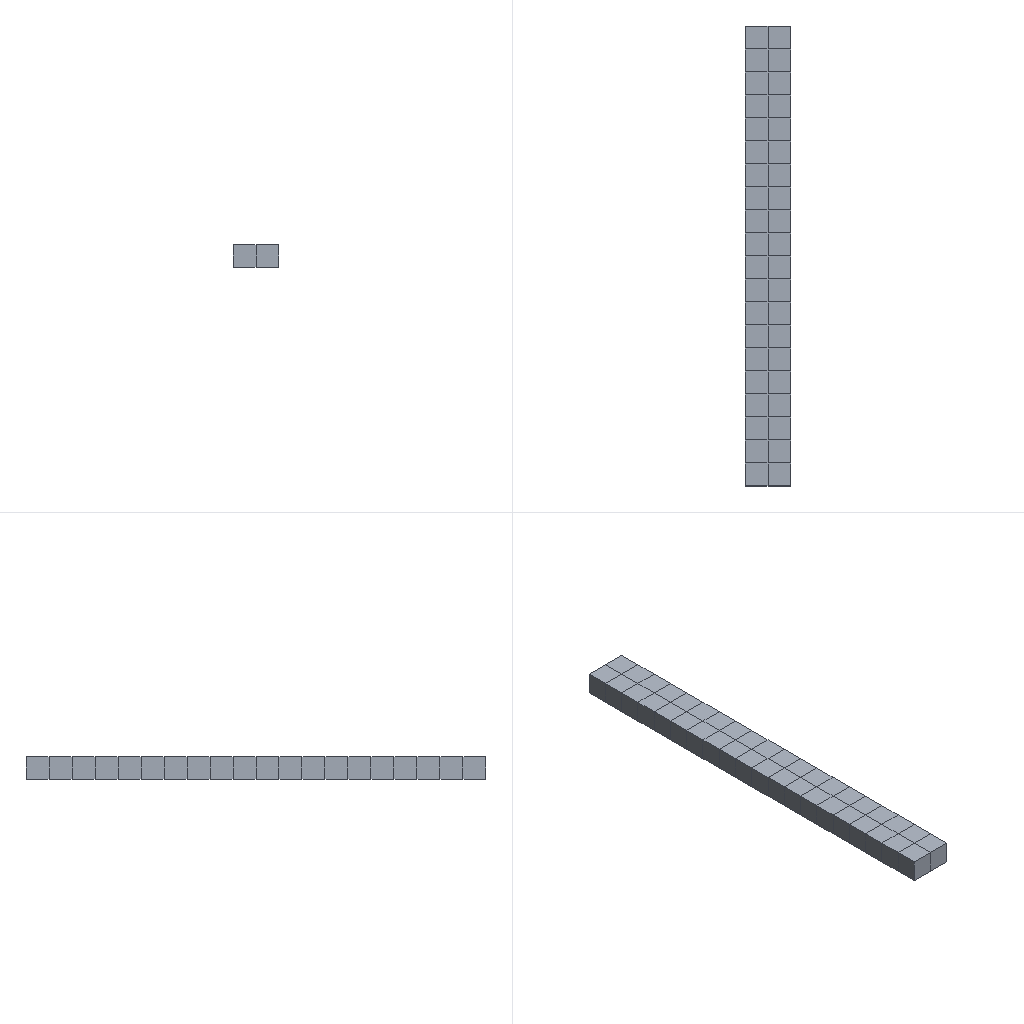Simulation study | ansys workbench
Set-up summary:
category,name,step,type,value,unit,region
solver,ansys_workbench
units,mm-N-s-tonne (MPa),,stated,"/units,MPA"
analysis,LS1,,static
load_step,LS1,LS1,static,nsubst=1; time=1
mesh,nodes,,,393
mesh,elements,,,41
element_type,SOLID186,,,40
element_type,SURF156,,,1
material,Structural Steel,,E,200000,tonne s^-2 mm^-1
material,Structural Steel,,nu,0.3
material,Structural Steel,,density,7.85e-09,tonne mm^-3
material,Structural Steel,,conductivity,60.5,tonne mm s^-3 C^-1
material,Structural Steel,,specific_heat,4.34e+08,mm^2 s^-2 C^-1
material,Structural Steel,,cte,1.2e-05,C^-1
material,Structural Steel,,permeability,10000
material,Structural Steel,,resistivity,0.00017,ohm mm
load,Define Force Using Surface Effect Elements,LS1,surface-effect pres face 1,200,,SURF156 #2
bc,Fixed Supports,model,fixed,[dofs=ALL],,_FIXEDSU
named_set,_FIXEDSU,,node,13
Ansys APDL input file, long lists of numbers shortened:
/batch
/config,noeldb,1     ! force off writing results to database
*get,_wallstrt,active,,time,wall
! ANSYS input file written by Workbench version 2022 R1
! File used for geometry attach:
/title,1--____ (C5)
! ****** Begin Custom Load Command Snippet ******
/COM, ACT Extensions:
/COM,     LSDYNA, 2021.1
/COM,
! ****** End   Custom Load Command Snippet ******
*DIM,_wb_ProjectScratch_dir,string,248
_wb_ProjectScratch_dir(1) = ''
*DIM,_wb_SolverFiles_dir,string,248
_wb_SolverFiles_dir(1) = ''
*DIM,_wb_userfiles_dir,string,248
_wb_userfiles_dir(1) = ''
/com,--- Data in consistent NMM units. See Solving Units in the help system for more information.
/units,MPA
/nopr
/wb,file,start              !  signify a WB generated input file
/prep7
! Turn off shape checking because checks already performed inside WB mesher.
! See help system for more information.
SHPP,OFF,,NOWARN
/nolist
etcon,set             ! allow ANSYS to choose best KEYOP's for 180x elements, resets any applicable keyopt to MAPDL defaults
/com,*********** Nodes for the whole assembly ***********
nblock,3,,432
(1i9,3e20.9e3)
        1     4.600000000E+01     5.000000000E+01    -2.500000000E+01
! (392 more lines like these left out)
-1
/wb,elem,start            !  set before creation of elements
/com,*********** Elements for Body 1 "SYS-2\__" ***********
et,1,186
keyo,1,2,1          ! set full integration on SOLID186
eblock,19,solid,,40
(19i9)
        1        1        1        1        0        0        0        0       20        0        1       19      125      124      122       20       40       41       42
! (79 more lines like these left out)
-1
/wb,elem,end               !  done creating elements
/com,*********** Send User Defined Coordinate System(s) ***********
csys,0
toffst,273.15,  ! Temperature offset from absolute zero
/com,*********** Set Reference Temperature ***********
tref,22.
/wb,mat,start              !  starting to send materials
/com,*********** Send Materials ***********
Temperature = 'TEMP' ! Temperature
MP,DENS,1,7.85e-09,	! tonne mm^-3
MP,ALPX,1,1.2e-05,	! C^-1
MP,C,1,434000000,	! mm^2 s^-2 C^-1
MP,KXX,1,60.5,	! tonne mm s^-3 C^-1
MP,RSVX,1,0.00017,	! ohm mm
MP,EX,1,200000,	! tonne s^-2 mm^-1
MP,NUXY,1,0.3,
MP,MURX,1,10000,
/wb,mat,end                !  done sending materials
!************************* Model Summary ********************
!SYS-2\__,	结构钢,	matid,	1
!************************* End Model Summary ********************
! get the diagonal of the bounding box. Needed later for other things
*get,_xmin,node,,mnloc,x
*get,_ymin,node,,mnloc,y
*get,_zmin,node,,mnloc,z
*get,_xmax,node,,mxloc,x
*get,_ymax,node,,mxloc,y
*get,_zmax,node,,mxloc,z
_ASMDIAG=(_xmax-_xmin)*(_xmax-_xmin)+(_ymax-_ymin)*(_ymax-_ymin)+(_zmax-_zmin)*(_zmax-_zmin)
_ASMDIAG=SQRT(_ASMDIAG)
/wb,contact,start          !  starting to send contact
/wb,contact,end            !  done creating contacts
/golist
/wb,load,start             !  starting to send loads
/com,*********** Fixed Supports ***********
CMBLOCK,_FIXEDSU,NODE,       13
(8i10)
        40        41        62       103       124       125       265       266
       267       269       310       371       393
cmsel,s,_FIXEDSU
d,all,all
nsel,all
/com,*********** Define Force Using Surface Effect Elements ***********
local,12,0,0.,0.,0.,0.,0.,0.
csys,0
et,2,156
keyop,2,5,1         !  No orientation node
eblock,10,,,1
(15i9)
      165        2        2        2       12      123       61      308
-1
esel,s,type,,2
keyop,2,2,1                ! Apply load in local coordinate system
keyop,2,7,1                ! Use original area so load is constant in large deformation
esel,all
/gst,on,on
fini
*get,_numnode,node,0,count
*get,_numelem,elem,0,count
*get, _MAXELEMNUM, elem, 0, NUM, MAX
*get, _MAXNODENUM, node, 0, NUM, MAX
*get, _MAXELEMTYPE, etyp, 0, NUM, MAX
*get, _MAXREALCONST, real, 0, NUM, MAX
/go
/wb,load,end               !  done creating loads
/com,--- Number of total nodes = %_numnode%
/com,--- Number of contact elements = 1
/com,--- Number of spring elements = 0
/com,--- Number of bearing elements = 0
/com,--- Number of solid elements = 40
/com,--- Number of condensed parts = 0
/com,--- Number of total elements = %_numelem%
*get,_wallbsol,active,,time,wall
/com,****************************************************************************
/com,*************************    SOLUTION       ********************************
/com,****************************************************************************
/solu
antype,0                   ! static analysis
_thickRatio=  0     ! Ratio of thick parts in the model
eqsl,sparse,,,,,1
cntr,print,1               ! print out contact info and also make no initial contact an error
dmpoption,emat,no             ! Don't combine emat file for DANSYS
dmpoption,esav,no             ! Don't combine esav file for DANSYS
nldiag,cont,iter           ! print out contact info each equilibrium iteration
rescontrol,,none                 ! Do not keep any restart files
/com,****************************************************
/com,******************* SOLVE FOR LS 1 OF 1 ****************
esel,s,type,,2
nsle
sfe,all,1,pres,1,200.
sfe,all,2,pres,1,0.
sfe,all,3,pres,1,0.
nsel,all
esel,all
/nopr
/gopr
nsub,1,1,1
time,1.
outres,erase
outres,all,none
outres,nsol,all,
outres,rsol,all
outres,eangl,all
outres,etmp,all
outres,veng,all
outres,strs,all,
outres,epel,all,
outres,eppl,all,
outres,cont,all,
! *********** WB SOLVE COMMAND ***********
! check interactive state
*get,ANSINTER_,active,,int
*if,ANSINTER_,ne,0,then
/eof
*endif
solve
/com *************** Write FE CONNECTORS *********
CEWRITE,file,ce,,INTE
/com,****************************************************
/com,*************** FINISHED SOLVE FOR LS 1 *************
*get,_wallasol,active,,time,wall
/nopr
*get,_numnode,node,0,count
*get,_numelem,elem,0,count
*get, _MAXELEMNUM, elem, 0, NUM, MAX
*get, _MAXNODENUM, node, 0, NUM, MAX,,,INTERNAL
*get, _MAXELEMTYPE, etyp, 0, NUM, MAX
*get, _MAXREALCONST, real, 0, NUM, MAX
/gopr
/post1
xmlo,ENCODING,ISO-8859-1
xmlo,parm
/xml,parm,xml
fini
/gopr
*get,_walldone,active,,time,wall
_preptime=(_wallbsol-_wallstrt)*3600
_solvtime=(_wallasol-_wallbsol)*3600
_posttime=(_walldone-_wallasol)*3600
_totaltim=(_walldone-_wallstrt)*3600
*get,_dlbratio,active,0,solu,dlbr
*get,_combtime,active,0,solu,comb
*get,_ssmode,active,0,solu,ssmm
*get,_ndofs,active,0,solu,ndof
*get,_sol_end_time,active,0,set,time
*if,_sol_end_time,eq,1.,then
/fclean				!clean distributed files
*endif
/com,--- Total number of nodes = %_numnode%
/com,--- Total number of elements = %_numelem%
/com,--- Element load balance ratio = %_dlbratio%
/com,--- Time to combine distributed files = %_combtime%
/com,--- Sparse memory mode = %_ssmode%
/com,--- Number of DOF = %_ndofs%
/wb,file,end               ! done with WB generated input
Results summary:
result,analyses[0].index,,,1
result,analyses[0].system,,,SYS-2
result,analyses[0].deck,,,deck.dat
result,analyses[0].solve_status,,,completed
result,analyses[0].analysis_type,,,static
result,analyses[0].physics,,,mechanical
result,analyses[0].unit_system,,,"NMM: mm, ton, N, s, mV, mA, degC"
result,analyses[0].n_sets,,,1
result,analyses[0].load_steps[0].set,set=1,,1
result,analyses[0].load_steps[0].time_or_freq,set=1,,1
result,analyses[0].load_steps[0].max_displacement_magnitude,set=1,,4.02
result,analyses[0].load_steps[0].max_von_mises_nodal,set=1,,121.38
result,analyses[0].load_steps[0].reaction_force_sum_xyz[1],set=1,,-10000
result,analyses[0].load_steps[0].reaction_force_sum_xyz[2],set=1,,1.07866e-07
result,analyses[0].load_steps[0].reaction_force_sum_xyz[3],set=1,,1.47192e-07
result,geometry_export[0][0],,,.step
result,geometry_export[0][1],,,ok
result,geometry_export[0][2],,,1